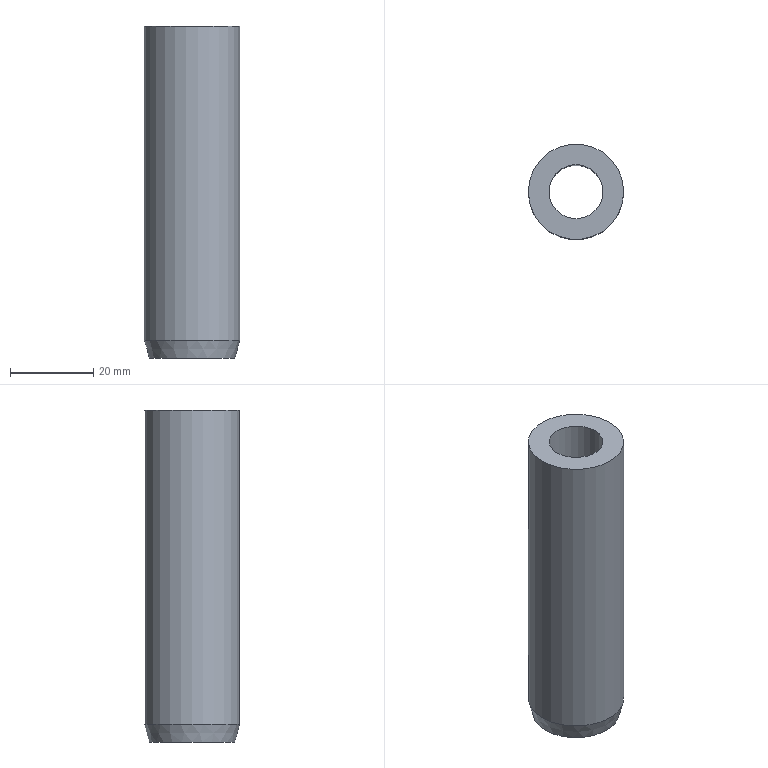Part | NX | features solid 2 | 1 solid | 5 faces | box 23 x 23 x 80 mm | volume 22449 mm3 | plane 2 | cylinder 2 | cone 1 | commonest cylinder face diameters 13 x1 23 x1
STEP:
#1=CARTESIAN_POINT('',(-143.5,70.,150.));
#2=VERTEX_POINT('',#1);
#3=CARTESIAN_POINT('',(-155.,70.,150.));
#4=DIRECTION('',(0.,0.,1.));
#5=DIRECTION('',(1.,0.,0.));
#6=AXIS2_PLACEMENT_3D('',#3,#4,#5);
#7=CIRCLE('',#6,11.5);
#8=EDGE_CURVE('',#2,#2,#7,.T.);
#9=ORIENTED_EDGE('',*,*,#8,.T.);
#10=EDGE_LOOP('',(#9));
#11=FACE_BOUND('',#10,.T.);
#12=CARTESIAN_POINT('',(-148.5,70.,150.));
#13=VERTEX_POINT('',#12);
#14=CARTESIAN_POINT('',(-155.,70.,150.));
#15=DIRECTION('',(0.,0.,1.));
#16=DIRECTION('',(1.,0.,0.));
#17=AXIS2_PLACEMENT_3D('',#14,#15,#16);
#18=CIRCLE('',#17,6.5);
#19=EDGE_CURVE('',#13,#13,#18,.T.);
#20=ORIENTED_EDGE('',*,*,#19,.F.);
#21=EDGE_LOOP('',(#20));
#22=FACE_BOUND('',#21,.T.);
#23=CARTESIAN_POINT('',(-155.,70.,150.));
#24=DIRECTION('',(0.,0.,1.));
#25=DIRECTION('',(1.,0.,0.));
#26=AXIS2_PLACEMENT_3D('',#23,#24,#25);
#27=PLANE('',#26);
#28=ADVANCED_FACE('',(#11,#22),#27,.T.);
#29=CARTESIAN_POINT('',(-144.644,70.,70.));
#30=VERTEX_POINT('',#29);
#31=CARTESIAN_POINT('',(-155.,70.,70.));
#32=DIRECTION('',(0.,0.,1.));
#33=DIRECTION('',(1.,0.,0.));
#34=AXIS2_PLACEMENT_3D('',#31,#32,#33);
#35=CIRCLE('',#34,10.356);
#36=EDGE_CURVE('',#30,#30,#35,.F.);
#37=ORIENTED_EDGE('',*,*,#36,.T.);
#38=EDGE_LOOP('',(#37));
#39=FACE_BOUND('',#38,.T.);
#40=CARTESIAN_POINT('',(-148.5,70.,70.));
#41=VERTEX_POINT('',#40);
#42=CARTESIAN_POINT('',(-155.,70.,70.));
#43=DIRECTION('',(0.,0.,1.));
#44=DIRECTION('',(1.,0.,0.));
#45=AXIS2_PLACEMENT_3D('',#42,#43,#44);
#46=CIRCLE('',#45,6.5);
#47=EDGE_CURVE('',#41,#41,#46,.T.);
#48=ORIENTED_EDGE('',*,*,#47,.T.);
#49=EDGE_LOOP('',(#48));
#50=FACE_BOUND('',#49,.T.);
#51=CARTESIAN_POINT('',(-155.,70.,70.));
#52=DIRECTION('',(0.,0.,1.));
#53=DIRECTION('',(1.,0.,0.));
#54=AXIS2_PLACEMENT_3D('',#51,#52,#53);
#55=PLANE('',#54);
#56=ADVANCED_FACE('',(#39,#50),#55,.F.);
#57=CARTESIAN_POINT('',(-143.5,70.,74.268));
#58=VERTEX_POINT('',#57);
#59=CARTESIAN_POINT('',(-155.,70.,74.268));
#60=DIRECTION('',(0.,0.,1.));
#61=DIRECTION('',(1.,0.,0.));
#62=AXIS2_PLACEMENT_3D('',#59,#60,#61);
#63=CIRCLE('',#62,11.5);
#64=EDGE_CURVE('',#58,#58,#63,.T.);
#65=ORIENTED_EDGE('',*,*,#64,.T.);
#66=EDGE_LOOP('',(#65));
#67=FACE_BOUND('',#66,.T.);
#68=ORIENTED_EDGE('',*,*,#8,.F.);
#69=EDGE_LOOP('',(#68));
#70=FACE_BOUND('',#69,.T.);
#71=CARTESIAN_POINT('',(-155.,70.,105.));
#72=DIRECTION('',(0.,0.,-1.));
#73=DIRECTION('',(-1.,0.,0.));
#74=AXIS2_PLACEMENT_3D('',#71,#72,#73);
#75=CYLINDRICAL_SURFACE('',#74,11.5);
#76=ADVANCED_FACE('',(#67,#70),#75,.T.);
#77=ORIENTED_EDGE('',*,*,#19,.T.);
#78=EDGE_LOOP('',(#77));
#79=FACE_BOUND('',#78,.T.);
#80=ORIENTED_EDGE('',*,*,#47,.F.);
#81=EDGE_LOOP('',(#80));
#82=FACE_BOUND('',#81,.T.);
#83=CARTESIAN_POINT('',(-155.,70.,105.));
#84=DIRECTION('',(0.,0.,-1.));
#85=DIRECTION('',(-1.,0.,0.));
#86=AXIS2_PLACEMENT_3D('',#83,#84,#85);
#87=CYLINDRICAL_SURFACE('',#86,6.5);
#88=ADVANCED_FACE('',(#79,#82),#87,.F.);
#89=ORIENTED_EDGE('',*,*,#36,.F.);
#90=EDGE_LOOP('',(#89));
#91=FACE_BOUND('',#90,.T.);
#92=ORIENTED_EDGE('',*,*,#64,.F.);
#93=EDGE_LOOP('',(#92));
#94=FACE_BOUND('',#93,.T.);
#95=CARTESIAN_POINT('',(-155.,70.,78.));
#96=DIRECTION('',(0.,0.,1.));
#97=DIRECTION('',(1.,0.,0.));
#98=AXIS2_PLACEMENT_3D('',#95,#96,#97);
#99=CONICAL_SURFACE('',#98,12.5,0.2618);
#100=ADVANCED_FACE('',(#91,#94),#99,.T.);
#101=CLOSED_SHELL('',(#28,#56,#76,#88,#100));
#102=MANIFOLD_SOLID_BREP('',#101);
#103=(LENGTH_UNIT()NAMED_UNIT(*)SI_UNIT(.MILLI.,.METRE.));
#104=UNCERTAINTY_MEASURE_WITH_UNIT(LENGTH_MEASURE(0.00001),#103,'','');
#105=(NAMED_UNIT(*)PLANE_ANGLE_UNIT()SI_UNIT($,.RADIAN.));
#106=(NAMED_UNIT(*)SI_UNIT($,.STERADIAN.)SOLID_ANGLE_UNIT());
#107=(GEOMETRIC_REPRESENTATION_CONTEXT(3)GLOBAL_UNCERTAINTY_ASSIGNED_CONTEXT((#104))GLOBAL_UNIT_ASSIGNED_CONTEXT((#103,#105,#106))REPRESENTATION_CONTEXT('',''));
#108=ADVANCED_BREP_SHAPE_REPRESENTATION('',(#102),#107);